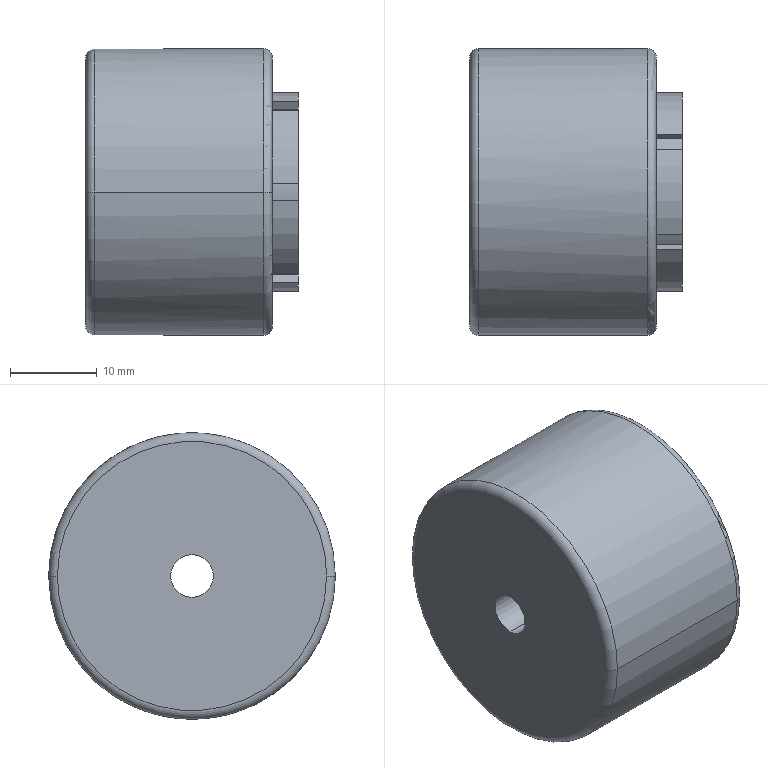Part | STEP file | ZUANZIWAITAO_4_1_2_1_1 | 1 solid | 38 faces | box 24.5 x 33 x 33 mm | volume 18261 mm3 | cylinder 18 | plane 16 | torus 4 | commonest cylinder face diameters 21 x6 23 x6 4.9 x2 17 x2 33 x2
STEP:
#1=CARTESIAN_POINT('',(0.,0.,0.));
#2=DIRECTION('',(0.,0.,1.));
#3=DIRECTION('',(1.,0.,0.));
#4=AXIS2_PLACEMENT_3D('',#1,#2,#3);
#5=CARTESIAN_POINT('',(0.,15.5,0.1054));
#6=VERTEX_POINT('',#5);
#7=CARTESIAN_POINT('',(0.,15.5,0.));
#8=VERTEX_POINT('',#7);
#9=CARTESIAN_POINT('',(0.,0.,0.));
#10=DIRECTION('',(-1.,0.,0.));
#11=DIRECTION('',(0.,1.,0.006802));
#12=AXIS2_PLACEMENT_3D('',#9,#10,#11);
#13=CIRCLE('',#12,15.5);
#14=EDGE_CURVE('',#6,#8,#13,.T.);
#15=ORIENTED_EDGE('',*,*,#14,.F.);
#16=CARTESIAN_POINT('',(0.,-15.5,0.));
#17=VERTEX_POINT('',#16);
#18=CARTESIAN_POINT('',(0.,0.,0.));
#19=DIRECTION('',(1.,0.,0.));
#20=DIRECTION('',(0.,1.,0.006802));
#21=AXIS2_PLACEMENT_3D('',#18,#19,#20);
#22=CIRCLE('',#21,15.5);
#23=EDGE_CURVE('',#6,#17,#22,.T.);
#24=ORIENTED_EDGE('',*,*,#23,.T.);
#25=CARTESIAN_POINT('',(0.,-15.5,-0.1054));
#26=VERTEX_POINT('',#25);
#27=CARTESIAN_POINT('',(0.,0.,0.));
#28=DIRECTION('',(-1.,0.,0.));
#29=DIRECTION('',(0.,-1.,-0.006802));
#30=AXIS2_PLACEMENT_3D('',#27,#28,#29);
#31=CIRCLE('',#30,15.5);
#32=EDGE_CURVE('',#26,#17,#31,.T.);
#33=ORIENTED_EDGE('',*,*,#32,.F.);
#34=CARTESIAN_POINT('',(0.,0.,0.));
#35=DIRECTION('',(1.,0.,0.));
#36=DIRECTION('',(0.,-1.,-0.006802));
#37=AXIS2_PLACEMENT_3D('',#34,#35,#36);
#38=CIRCLE('',#37,15.5);
#39=EDGE_CURVE('',#26,#8,#38,.T.);
#40=ORIENTED_EDGE('',*,*,#39,.T.);
#41=EDGE_LOOP('',(#15,#24,#33,#40));
#42=FACE_OUTER_BOUND('',#41,.F.);
#43=CARTESIAN_POINT('',(0.,0.,2.45));
#44=VERTEX_POINT('',#43);
#45=CARTESIAN_POINT('',(0.,0.,-2.45));
#46=VERTEX_POINT('',#45);
#47=CARTESIAN_POINT('',(0.,0.,0.));
#48=DIRECTION('',(-1.,0.,0.));
#49=DIRECTION('',(0.,0.,1.));
#50=AXIS2_PLACEMENT_3D('',#47,#48,#49);
#51=CIRCLE('',#50,2.45);
#52=EDGE_CURVE('',#44,#46,#51,.T.);
#53=ORIENTED_EDGE('',*,*,#52,.T.);
#54=CARTESIAN_POINT('',(0.,0.,0.));
#55=DIRECTION('',(-1.,0.,0.));
#56=DIRECTION('',(0.,0.,-1.));
#57=AXIS2_PLACEMENT_3D('',#54,#55,#56);
#58=CIRCLE('',#57,2.45);
#59=EDGE_CURVE('',#46,#44,#58,.T.);
#60=ORIENTED_EDGE('',*,*,#59,.T.);
#61=EDGE_LOOP('',(#53,#60));
#62=FACE_BOUND('',#61,.F.);
#63=CARTESIAN_POINT('',(0.,0.,0.));
#64=DIRECTION('',(1.,0.,0.));
#65=DIRECTION('',(0.,-1.,0.));
#66=AXIS2_PLACEMENT_3D('',#63,#64,#65);
#67=PLANE('',#66);
#68=ADVANCED_FACE('',(#42,#62),#67,.F.);
#69=ORIENTED_EDGE('',*,*,#23,.F.);
#70=ORIENTED_EDGE('',*,*,#14,.T.);
#71=CARTESIAN_POINT('',(1.,16.5,0.));
#72=VERTEX_POINT('',#71);
#73=CARTESIAN_POINT('',(1.,15.5,0.));
#74=DIRECTION('',(0.,0.,-1.));
#75=DIRECTION('',(-1.,0.,0.));
#76=AXIS2_PLACEMENT_3D('',#73,#74,#75);
#77=CIRCLE('',#76,1.);
#78=EDGE_CURVE('',#8,#72,#77,.T.);
#79=ORIENTED_EDGE('',*,*,#78,.T.);
#80=CARTESIAN_POINT('',(1.,16.5,0.1122));
#81=VERTEX_POINT('',#80);
#82=CARTESIAN_POINT('',(1.,0.,0.));
#83=DIRECTION('',(1.,0.,0.));
#84=DIRECTION('',(0.,1.,0.));
#85=AXIS2_PLACEMENT_3D('',#82,#83,#84);
#86=CIRCLE('',#85,16.5);
#87=EDGE_CURVE('',#72,#81,#86,.T.);
#88=ORIENTED_EDGE('',*,*,#87,.T.);
#89=CARTESIAN_POINT('',(1.,-16.5,0.));
#90=VERTEX_POINT('',#89);
#91=CARTESIAN_POINT('',(1.,0.,0.));
#92=DIRECTION('',(1.,0.,0.));
#93=DIRECTION('',(0.,1.,0.006802));
#94=AXIS2_PLACEMENT_3D('',#91,#92,#93);
#95=CIRCLE('',#94,16.5);
#96=EDGE_CURVE('',#81,#90,#95,.T.);
#97=ORIENTED_EDGE('',*,*,#96,.T.);
#98=CARTESIAN_POINT('',(1.,-15.5,0.));
#99=DIRECTION('',(0.,0.,1.));
#100=DIRECTION('',(-1.,0.,0.));
#101=AXIS2_PLACEMENT_3D('',#98,#99,#100);
#102=CIRCLE('',#101,1.);
#103=EDGE_CURVE('',#17,#90,#102,.T.);
#104=ORIENTED_EDGE('',*,*,#103,.F.);
#105=EDGE_LOOP('',(#69,#70,#79,#88,#97,#104));
#106=FACE_OUTER_BOUND('',#105,.F.);
#107=CARTESIAN_POINT('',(1.,0.,0.));
#108=DIRECTION('',(1.,0.,0.));
#109=DIRECTION('',(0.,-1.,-0.006802));
#110=AXIS2_PLACEMENT_3D('',#107,#108,#109);
#111=TOROIDAL_SURFACE('',#110,15.5,1.);
#112=ADVANCED_FACE('',(#106),#111,.T.);
#113=ORIENTED_EDGE('',*,*,#39,.F.);
#114=ORIENTED_EDGE('',*,*,#32,.T.);
#115=ORIENTED_EDGE('',*,*,#103,.T.);
#116=CARTESIAN_POINT('',(1.,-16.5,-0.1122));
#117=VERTEX_POINT('',#116);
#118=CARTESIAN_POINT('',(1.,0.,0.));
#119=DIRECTION('',(1.,0.,0.));
#120=DIRECTION('',(0.,-1.,0.));
#121=AXIS2_PLACEMENT_3D('',#118,#119,#120);
#122=CIRCLE('',#121,16.5);
#123=EDGE_CURVE('',#90,#117,#122,.T.);
#124=ORIENTED_EDGE('',*,*,#123,.T.);
#125=CARTESIAN_POINT('',(1.,0.,0.));
#126=DIRECTION('',(1.,0.,0.));
#127=DIRECTION('',(0.,-1.,-0.006802));
#128=AXIS2_PLACEMENT_3D('',#125,#126,#127);
#129=CIRCLE('',#128,16.5);
#130=EDGE_CURVE('',#117,#72,#129,.T.);
#131=ORIENTED_EDGE('',*,*,#130,.T.);
#132=ORIENTED_EDGE('',*,*,#78,.F.);
#133=EDGE_LOOP('',(#113,#114,#115,#124,#131,#132));
#134=FACE_OUTER_BOUND('',#133,.F.);
#135=CARTESIAN_POINT('',(1.,0.,0.));
#136=DIRECTION('',(1.,0.,0.));
#137=DIRECTION('',(0.,1.,0.006802));
#138=AXIS2_PLACEMENT_3D('',#135,#136,#137);
#139=TOROIDAL_SURFACE('',#138,15.5,1.);
#140=ADVANCED_FACE('',(#134),#139,.T.);
#141=CARTESIAN_POINT('',(20.5,16.5,-0.07901));
#142=VERTEX_POINT('',#141);
#143=CARTESIAN_POINT('',(20.5,-16.5,0.));
#144=VERTEX_POINT('',#143);
#145=CARTESIAN_POINT('',(20.5,0.,0.));
#146=DIRECTION('',(-1.,0.,0.));
#147=DIRECTION('',(0.,1.,-0.004788));
#148=AXIS2_PLACEMENT_3D('',#145,#146,#147);
#149=CIRCLE('',#148,16.5);
#150=EDGE_CURVE('',#142,#144,#149,.T.);
#151=ORIENTED_EDGE('',*,*,#150,.F.);
#152=CARTESIAN_POINT('',(20.5,16.5,0.));
#153=VERTEX_POINT('',#152);
#154=CARTESIAN_POINT('',(20.5,0.,0.));
#155=DIRECTION('',(-1.,0.,0.));
#156=DIRECTION('',(0.,1.,0.));
#157=AXIS2_PLACEMENT_3D('',#154,#155,#156);
#158=CIRCLE('',#157,16.5);
#159=EDGE_CURVE('',#153,#142,#158,.T.);
#160=ORIENTED_EDGE('',*,*,#159,.F.);
#161=CARTESIAN_POINT('',(1.,16.5,0.));
#162=DIRECTION('',(1.,0.,0.));
#163=VECTOR('',#162,19.5);
#164=LINE('',#161,#163);
#165=EDGE_CURVE('',#72,#153,#164,.T.);
#166=ORIENTED_EDGE('',*,*,#165,.F.);
#167=ORIENTED_EDGE('',*,*,#130,.F.);
#168=ORIENTED_EDGE('',*,*,#123,.F.);
#169=CARTESIAN_POINT('',(1.,-16.5,0.));
#170=DIRECTION('',(1.,0.,0.));
#171=VECTOR('',#170,19.5);
#172=LINE('',#169,#171);
#173=EDGE_CURVE('',#90,#144,#172,.T.);
#174=ORIENTED_EDGE('',*,*,#173,.T.);
#175=EDGE_LOOP('',(#151,#160,#166,#167,#168,#174));
#176=FACE_OUTER_BOUND('',#175,.F.);
#177=CARTESIAN_POINT('',(0.,0.,0.));
#178=DIRECTION('',(1.,0.,0.));
#179=DIRECTION('',(0.,-1.,0.));
#180=AXIS2_PLACEMENT_3D('',#177,#178,#179);
#181=CYLINDRICAL_SURFACE('',#180,16.5);
#182=ADVANCED_FACE('',(#176),#181,.T.);
#183=CARTESIAN_POINT('',(21.5,15.5,-0.07422));
#184=VERTEX_POINT('',#183);
#185=CARTESIAN_POINT('',(21.5,-15.5,0.));
#186=VERTEX_POINT('',#185);
#187=CARTESIAN_POINT('',(21.5,0.,0.));
#188=DIRECTION('',(-1.,0.,0.));
#189=DIRECTION('',(0.,1.,-0.004788));
#190=AXIS2_PLACEMENT_3D('',#187,#188,#189);
#191=CIRCLE('',#190,15.5);
#192=EDGE_CURVE('',#184,#186,#191,.T.);
#193=ORIENTED_EDGE('',*,*,#192,.F.);
#194=CARTESIAN_POINT('',(21.5,15.5,0.));
#195=VERTEX_POINT('',#194);
#196=CARTESIAN_POINT('',(21.5,0.,0.));
#197=DIRECTION('',(1.,0.,0.));
#198=DIRECTION('',(0.,1.,-0.004788));
#199=AXIS2_PLACEMENT_3D('',#196,#197,#198);
#200=CIRCLE('',#199,15.5);
#201=EDGE_CURVE('',#184,#195,#200,.T.);
#202=ORIENTED_EDGE('',*,*,#201,.T.);
#203=CARTESIAN_POINT('',(20.5,15.5,0.));
#204=DIRECTION('',(0.,0.,1.));
#205=DIRECTION('',(1.,0.,0.));
#206=AXIS2_PLACEMENT_3D('',#203,#204,#205);
#207=CIRCLE('',#206,1.);
#208=EDGE_CURVE('',#195,#153,#207,.T.);
#209=ORIENTED_EDGE('',*,*,#208,.T.);
#210=ORIENTED_EDGE('',*,*,#159,.T.);
#211=ORIENTED_EDGE('',*,*,#150,.T.);
#212=CARTESIAN_POINT('',(20.5,-15.5,0.));
#213=DIRECTION('',(0.,0.,-1.));
#214=DIRECTION('',(1.,0.,0.));
#215=AXIS2_PLACEMENT_3D('',#212,#213,#214);
#216=CIRCLE('',#215,1.);
#217=EDGE_CURVE('',#186,#144,#216,.T.);
#218=ORIENTED_EDGE('',*,*,#217,.F.);
#219=EDGE_LOOP('',(#193,#202,#209,#210,#211,#218));
#220=FACE_OUTER_BOUND('',#219,.F.);
#221=CARTESIAN_POINT('',(20.5,0.,0.));
#222=DIRECTION('',(1.,0.,0.));
#223=DIRECTION('',(0.,-1.,0.004788));
#224=AXIS2_PLACEMENT_3D('',#221,#222,#223);
#225=TOROIDAL_SURFACE('',#224,15.5,1.);
#226=ADVANCED_FACE('',(#220),#225,.T.);
#227=CARTESIAN_POINT('',(21.5,-15.5,0.07422));
#228=VERTEX_POINT('',#227);
#229=CARTESIAN_POINT('',(21.5,0.,0.));
#230=DIRECTION('',(1.,0.,0.));
#231=DIRECTION('',(0.,-1.,0.004788));
#232=AXIS2_PLACEMENT_3D('',#229,#230,#231);
#233=CIRCLE('',#232,15.5);
#234=EDGE_CURVE('',#228,#186,#233,.T.);
#235=ORIENTED_EDGE('',*,*,#234,.F.);
#236=CARTESIAN_POINT('',(21.5,0.,0.));
#237=DIRECTION('',(-1.,0.,0.));
#238=DIRECTION('',(0.,-1.,0.004788));
#239=AXIS2_PLACEMENT_3D('',#236,#237,#238);
#240=CIRCLE('',#239,15.5);
#241=EDGE_CURVE('',#228,#195,#240,.T.);
#242=ORIENTED_EDGE('',*,*,#241,.T.);
#243=ORIENTED_EDGE('',*,*,#201,.F.);
#244=ORIENTED_EDGE('',*,*,#192,.T.);
#245=EDGE_LOOP('',(#235,#242,#243,#244));
#246=FACE_OUTER_BOUND('',#245,.F.);
#247=CARTESIAN_POINT('',(21.5,-6.594,9.422));
#248=VERTEX_POINT('',#247);
#249=CARTESIAN_POINT('',(21.5,-11.456,1.));
#250=VERTEX_POINT('',#249);
#251=CARTESIAN_POINT('',(21.5,0.,0.));
#252=DIRECTION('',(1.,0.,0.));
#253=DIRECTION('',(0.,-0.5734,0.8193));
#254=AXIS2_PLACEMENT_3D('',#251,#252,#253);
#255=CIRCLE('',#254,11.5);
#256=EDGE_CURVE('',#248,#250,#255,.T.);
#257=ORIENTED_EDGE('',*,*,#256,.T.);
#258=CARTESIAN_POINT('',(21.5,-10.452,1.));
#259=VERTEX_POINT('',#258);
#260=CARTESIAN_POINT('',(21.5,-10.452,1.));
#261=DIRECTION('',(0.,-1.,0.));
#262=VECTOR('',#261,1.004);
#263=LINE('',#260,#262);
#264=EDGE_CURVE('',#259,#250,#263,.T.);
#265=ORIENTED_EDGE('',*,*,#264,.F.);
#266=CARTESIAN_POINT('',(21.5,-10.452,-1.));
#267=VERTEX_POINT('',#266);
#268=CARTESIAN_POINT('',(21.5,0.,0.));
#269=DIRECTION('',(1.,0.,0.));
#270=DIRECTION('',(0.,-0.9955,0.09524));
#271=AXIS2_PLACEMENT_3D('',#268,#269,#270);
#272=CIRCLE('',#271,10.5);
#273=EDGE_CURVE('',#259,#267,#272,.T.);
#274=ORIENTED_EDGE('',*,*,#273,.T.);
#275=CARTESIAN_POINT('',(21.5,-11.456,-1.));
#276=VERTEX_POINT('',#275);
#277=CARTESIAN_POINT('',(21.5,-11.456,-1.));
#278=DIRECTION('',(0.,1.,0.));
#279=VECTOR('',#278,1.004);
#280=LINE('',#277,#279);
#281=EDGE_CURVE('',#276,#267,#280,.T.);
#282=ORIENTED_EDGE('',*,*,#281,.F.);
#283=CARTESIAN_POINT('',(21.5,-6.594,-9.422));
#284=VERTEX_POINT('',#283);
#285=CARTESIAN_POINT('',(21.5,0.,0.));
#286=DIRECTION('',(1.,0.,0.));
#287=DIRECTION('',(0.,-0.9962,-0.08696));
#288=AXIS2_PLACEMENT_3D('',#285,#286,#287);
#289=CIRCLE('',#288,11.5);
#290=EDGE_CURVE('',#276,#284,#289,.T.);
#291=ORIENTED_EDGE('',*,*,#290,.T.);
#292=CARTESIAN_POINT('',(21.5,-6.092,-8.552));
#293=VERTEX_POINT('',#292);
#294=CARTESIAN_POINT('',(21.5,-6.594,-9.422));
#295=DIRECTION('',(0.,0.5,0.866));
#296=VECTOR('',#295,1.004);
#297=LINE('',#294,#296);
#298=EDGE_CURVE('',#284,#293,#297,.T.);
#299=ORIENTED_EDGE('',*,*,#298,.T.);
#300=CARTESIAN_POINT('',(21.5,-4.36,-9.552));
#301=VERTEX_POINT('',#300);
#302=CARTESIAN_POINT('',(21.5,0.,0.));
#303=DIRECTION('',(1.,0.,0.));
#304=DIRECTION('',(0.,-0.5802,-0.8145));
#305=AXIS2_PLACEMENT_3D('',#302,#303,#304);
#306=CIRCLE('',#305,10.5);
#307=EDGE_CURVE('',#293,#301,#306,.T.);
#308=ORIENTED_EDGE('',*,*,#307,.T.);
#309=CARTESIAN_POINT('',(21.5,-4.862,-10.422));
#310=VERTEX_POINT('',#309);
#311=CARTESIAN_POINT('',(21.5,-4.36,-9.552));
#312=DIRECTION('',(0.,-0.5,-0.866));
#313=VECTOR('',#312,1.004);
#314=LINE('',#311,#313);
#315=EDGE_CURVE('',#301,#310,#314,.T.);
#316=ORIENTED_EDGE('',*,*,#315,.T.);
#317=CARTESIAN_POINT('',(21.5,4.862,-10.422));
#318=VERTEX_POINT('',#317);
#319=CARTESIAN_POINT('',(21.5,0.,0.));
#320=DIRECTION('',(1.,0.,0.));
#321=DIRECTION('',(0.,-0.4228,-0.9062));
#322=AXIS2_PLACEMENT_3D('',#319,#320,#321);
#323=CIRCLE('',#322,11.5);
#324=EDGE_CURVE('',#310,#318,#323,.T.);
#325=ORIENTED_EDGE('',*,*,#324,.T.);
#326=CARTESIAN_POINT('',(21.5,4.36,-9.552));
#327=VERTEX_POINT('',#326);
#328=CARTESIAN_POINT('',(21.5,4.862,-10.422));
#329=DIRECTION('',(0.,-0.5,0.866));
#330=VECTOR('',#329,1.004);
#331=LINE('',#328,#330);
#332=EDGE_CURVE('',#318,#327,#331,.T.);
#333=ORIENTED_EDGE('',*,*,#332,.T.);
#334=CARTESIAN_POINT('',(21.5,6.092,-8.552));
#335=VERTEX_POINT('',#334);
#336=CARTESIAN_POINT('',(21.5,0.,0.));
#337=DIRECTION('',(1.,0.,0.));
#338=DIRECTION('',(0.,0.4152,-0.9097));
#339=AXIS2_PLACEMENT_3D('',#336,#337,#338);
#340=CIRCLE('',#339,10.5);
#341=EDGE_CURVE('',#327,#335,#340,.T.);
#342=ORIENTED_EDGE('',*,*,#341,.T.);
#343=CARTESIAN_POINT('',(21.5,6.594,-9.422));
#344=VERTEX_POINT('',#343);
#345=CARTESIAN_POINT('',(21.5,6.092,-8.552));
#346=DIRECTION('',(0.,0.5,-0.866));
#347=VECTOR('',#346,1.004);
#348=LINE('',#345,#347);
#349=EDGE_CURVE('',#335,#344,#348,.T.);
#350=ORIENTED_EDGE('',*,*,#349,.T.);
#351=CARTESIAN_POINT('',(21.5,11.456,-1.));
#352=VERTEX_POINT('',#351);
#353=CARTESIAN_POINT('',(21.5,0.,0.));
#354=DIRECTION('',(1.,0.,0.));
#355=DIRECTION('',(0.,0.5734,-0.8193));
#356=AXIS2_PLACEMENT_3D('',#353,#354,#355);
#357=CIRCLE('',#356,11.5);
#358=EDGE_CURVE('',#344,#352,#357,.T.);
#359=ORIENTED_EDGE('',*,*,#358,.T.);
#360=CARTESIAN_POINT('',(21.5,10.452,-1.));
#361=VERTEX_POINT('',#360);
#362=CARTESIAN_POINT('',(21.5,10.452,-1.));
#363=DIRECTION('',(0.,1.,0.));
#364=VECTOR('',#363,1.004);
#365=LINE('',#362,#364);
#366=EDGE_CURVE('',#361,#352,#365,.T.);
#367=ORIENTED_EDGE('',*,*,#366,.F.);
#368=CARTESIAN_POINT('',(21.5,10.452,1.));
#369=VERTEX_POINT('',#368);
#370=CARTESIAN_POINT('',(21.5,0.,0.));
#371=DIRECTION('',(1.,0.,0.));
#372=DIRECTION('',(0.,0.9955,-0.09524));
#373=AXIS2_PLACEMENT_3D('',#370,#371,#372);
#374=CIRCLE('',#373,10.5);
#375=EDGE_CURVE('',#361,#369,#374,.T.);
#376=ORIENTED_EDGE('',*,*,#375,.T.);
#377=CARTESIAN_POINT('',(21.5,11.456,1.));
#378=VERTEX_POINT('',#377);
#379=CARTESIAN_POINT('',(21.5,11.456,1.));
#380=DIRECTION('',(0.,-1.,0.));
#381=VECTOR('',#380,1.004);
#382=LINE('',#379,#381);
#383=EDGE_CURVE('',#378,#369,#382,.T.);
#384=ORIENTED_EDGE('',*,*,#383,.F.);
#385=CARTESIAN_POINT('',(21.5,6.594,9.422));
#386=VERTEX_POINT('',#385);
#387=CARTESIAN_POINT('',(21.5,0.,0.));
#388=DIRECTION('',(1.,0.,0.));
#389=DIRECTION('',(0.,0.9962,0.08696));
#390=AXIS2_PLACEMENT_3D('',#387,#388,#389);
#391=CIRCLE('',#390,11.5);
#392=EDGE_CURVE('',#378,#386,#391,.T.);
#393=ORIENTED_EDGE('',*,*,#392,.T.);
#394=CARTESIAN_POINT('',(21.5,6.092,8.552));
#395=VERTEX_POINT('',#394);
#396=CARTESIAN_POINT('',(21.5,6.594,9.422));
#397=DIRECTION('',(0.,-0.5,-0.866));
#398=VECTOR('',#397,1.004);
#399=LINE('',#396,#398);
#400=EDGE_CURVE('',#386,#395,#399,.T.);
#401=ORIENTED_EDGE('',*,*,#400,.T.);
#402=CARTESIAN_POINT('',(21.5,4.36,9.552));
#403=VERTEX_POINT('',#402);
#404=CARTESIAN_POINT('',(21.5,0.,0.));
#405=DIRECTION('',(1.,0.,0.));
#406=DIRECTION('',(0.,0.5802,0.8145));
#407=AXIS2_PLACEMENT_3D('',#404,#405,#406);
#408=CIRCLE('',#407,10.5);
#409=EDGE_CURVE('',#395,#403,#408,.T.);
#410=ORIENTED_EDGE('',*,*,#409,.T.);
#411=CARTESIAN_POINT('',(21.5,4.862,10.422));
#412=VERTEX_POINT('',#411);
#413=CARTESIAN_POINT('',(21.5,4.36,9.552));
#414=DIRECTION('',(0.,0.5,0.866));
#415=VECTOR('',#414,1.004);
#416=LINE('',#413,#415);
#417=EDGE_CURVE('',#403,#412,#416,.T.);
#418=ORIENTED_EDGE('',*,*,#417,.T.);
#419=CARTESIAN_POINT('',(21.5,-4.862,10.422));
#420=VERTEX_POINT('',#419);
#421=CARTESIAN_POINT('',(21.5,0.,0.));
#422=DIRECTION('',(1.,0.,0.));
#423=DIRECTION('',(0.,0.4228,0.9062));
#424=AXIS2_PLACEMENT_3D('',#421,#422,#423);
#425=CIRCLE('',#424,11.5);
#426=EDGE_CURVE('',#412,#420,#425,.T.);
#427=ORIENTED_EDGE('',*,*,#426,.T.);
#428=CARTESIAN_POINT('',(21.5,-4.36,9.552));
#429=VERTEX_POINT('',#428);
#430=CARTESIAN_POINT('',(21.5,-4.862,10.422));
#431=DIRECTION('',(0.,0.5,-0.866));
#432=VECTOR('',#431,1.004);
#433=LINE('',#430,#432);
#434=EDGE_CURVE('',#420,#429,#433,.T.);
#435=ORIENTED_EDGE('',*,*,#434,.T.);
#436=CARTESIAN_POINT('',(21.5,-6.092,8.552));
#437=VERTEX_POINT('',#436);
#438=CARTESIAN_POINT('',(21.5,0.,0.));
#439=DIRECTION('',(1.,0.,0.));
#440=DIRECTION('',(0.,-0.4152,0.9097));
#441=AXIS2_PLACEMENT_3D('',#438,#439,#440);
#442=CIRCLE('',#441,10.5);
#443=EDGE_CURVE('',#429,#437,#442,.T.);
#444=ORIENTED_EDGE('',*,*,#443,.T.);
#445=CARTESIAN_POINT('',(21.5,-6.092,8.552));
#446=DIRECTION('',(0.,-0.5,0.866));
#447=VECTOR('',#446,1.004);
#448=LINE('',#445,#447);
#449=EDGE_CURVE('',#437,#248,#448,.T.);
#450=ORIENTED_EDGE('',*,*,#449,.T.);
#451=EDGE_LOOP('',(#257,#265,#274,#282,#291,#299,#308,#316,#325,#333,#342,#350,#359,#367,#376,#384,#393,#401,#410,#418,#427,#435,#444,#450));
#452=FACE_BOUND('',#451,.F.);
#453=CARTESIAN_POINT('',(21.5,0.,0.));
#454=DIRECTION('',(1.,0.,0.));
#455=DIRECTION('',(0.,-1.,0.));
#456=AXIS2_PLACEMENT_3D('',#453,#454,#455);
#457=PLANE('',#456);
#458=ADVANCED_FACE('',(#246,#452),#457,.T.);
#459=ORIENTED_EDGE('',*,*,#241,.F.);
#460=ORIENTED_EDGE('',*,*,#234,.T.);
#461=ORIENTED_EDGE('',*,*,#217,.T.);
#462=CARTESIAN_POINT('',(20.5,-16.5,0.07901));
#463=VERTEX_POINT('',#462);
#464=CARTESIAN_POINT('',(20.5,0.,0.));
#465=DIRECTION('',(-1.,0.,0.));
#466=DIRECTION('',(0.,-1.,0.));
#467=AXIS2_PLACEMENT_3D('',#464,#465,#466);
#468=CIRCLE('',#467,16.5);
#469=EDGE_CURVE('',#144,#463,#468,.T.);
#470=ORIENTED_EDGE('',*,*,#469,.T.);
#471=CARTESIAN_POINT('',(20.5,0.,0.));
#472=DIRECTION('',(-1.,0.,0.));
#473=DIRECTION('',(0.,-1.,0.004788));
#474=AXIS2_PLACEMENT_3D('',#471,#472,#473);
#475=CIRCLE('',#474,16.5);
#476=EDGE_CURVE('',#463,#153,#475,.T.);
#477=ORIENTED_EDGE('',*,*,#476,.T.);
#478=ORIENTED_EDGE('',*,*,#208,.F.);
#479=EDGE_LOOP('',(#459,#460,#461,#470,#477,#478));
#480=FACE_OUTER_BOUND('',#479,.F.);
#481=CARTESIAN_POINT('',(20.5,0.,0.));
#482=DIRECTION('',(1.,0.,0.));
#483=DIRECTION('',(0.,1.,-0.004788));
#484=AXIS2_PLACEMENT_3D('',#481,#482,#483);
#485=TOROIDAL_SURFACE('',#484,15.5,1.);
#486=ADVANCED_FACE('',(#480),#485,.T.);
#487=ORIENTED_EDGE('',*,*,#476,.F.);
#488=ORIENTED_EDGE('',*,*,#469,.F.);
#489=ORIENTED_EDGE('',*,*,#173,.F.);
#490=ORIENTED_EDGE('',*,*,#96,.F.);
#491=ORIENTED_EDGE('',*,*,#87,.F.);
#492=ORIENTED_EDGE('',*,*,#165,.T.);
#493=EDGE_LOOP('',(#487,#488,#489,#490,#491,#492));
#494=FACE_OUTER_BOUND('',#493,.F.);
#495=CARTESIAN_POINT('',(0.,0.,0.));
#496=DIRECTION('',(1.,0.,0.));
#497=DIRECTION('',(0.,-1.,0.));
#498=AXIS2_PLACEMENT_3D('',#495,#496,#497);
#499=CYLINDRICAL_SURFACE('',#498,16.5);
#500=ADVANCED_FACE('',(#494),#499,.T.);
#501=CARTESIAN_POINT('',(24.5,-11.456,1.));
#502=VERTEX_POINT('',#501);
#503=CARTESIAN_POINT('',(24.5,-11.456,1.));
#504=DIRECTION('',(-1.,0.,0.));
#505=VECTOR('',#504,3.);
#506=LINE('',#503,#505);
#507=EDGE_CURVE('',#502,#250,#506,.T.);
#508=ORIENTED_EDGE('',*,*,#507,.T.);
#509=ORIENTED_EDGE('',*,*,#256,.F.);
#510=CARTESIAN_POINT('',(24.5,-6.594,9.422));
#511=VERTEX_POINT('',#510);
#512=CARTESIAN_POINT('',(21.5,-6.594,9.422));
#513=DIRECTION('',(1.,0.,0.));
#514=VECTOR('',#513,3.);
#515=LINE('',#512,#514);
#516=EDGE_CURVE('',#248,#511,#515,.T.);
#517=ORIENTED_EDGE('',*,*,#516,.T.);
#518=CARTESIAN_POINT('',(24.5,0.,0.));
#519=DIRECTION('',(-1.,0.,0.));
#520=DIRECTION('',(0.,-0.9962,0.08696));
#521=AXIS2_PLACEMENT_3D('',#518,#519,#520);
#522=CIRCLE('',#521,11.5);
#523=EDGE_CURVE('',#502,#511,#522,.T.);
#524=ORIENTED_EDGE('',*,*,#523,.F.);
#525=EDGE_LOOP('',(#508,#509,#517,#524));
#526=FACE_OUTER_BOUND('',#525,.F.);
#527=CARTESIAN_POINT('',(21.5,0.,0.));
#528=DIRECTION('',(1.,0.,0.));
#529=DIRECTION('',(0.,-1.,0.));
#530=AXIS2_PLACEMENT_3D('',#527,#528,#529);
#531=CYLINDRICAL_SURFACE('',#530,11.5);
#532=ADVANCED_FACE('',(#526),#531,.T.);
#533=CARTESIAN_POINT('',(24.5,-10.452,1.));
#534=VERTEX_POINT('',#533);
#535=CARTESIAN_POINT('',(24.5,-10.452,1.));
#536=DIRECTION('',(0.,-1.,0.));
#537=VECTOR('',#536,1.004);
#538=LINE('',#535,#537);
#539=EDGE_CURVE('',#534,#502,#538,.T.);
#540=ORIENTED_EDGE('',*,*,#539,.F.);
#541=CARTESIAN_POINT('',(21.5,-10.452,1.));
#542=DIRECTION('',(1.,0.,0.));
#543=VECTOR('',#542,3.);
#544=LINE('',#541,#543);
#545=EDGE_CURVE('',#259,#534,#544,.T.);
#546=ORIENTED_EDGE('',*,*,#545,.F.);
#547=ORIENTED_EDGE('',*,*,#264,.T.);
#548=ORIENTED_EDGE('',*,*,#507,.F.);
#549=EDGE_LOOP('',(#540,#546,#547,#548));
#550=FACE_OUTER_BOUND('',#549,.F.);
#551=CARTESIAN_POINT('',(24.5,-10.452,1.));
#552=DIRECTION('',(0.,0.,1.));
#553=DIRECTION('',(0.,-1.,0.));
#554=AXIS2_PLACEMENT_3D('',#551,#552,#553);
#555=PLANE('',#554);
#556=ADVANCED_FACE('',(#550),#555,.F.);
#557=CARTESIAN_POINT('',(24.5,-11.456,-1.));
#558=VERTEX_POINT('',#557);
#559=CARTESIAN_POINT('',(24.5,-10.452,-1.));
#560=VERTEX_POINT('',#559);
#561=CARTESIAN_POINT('',(24.5,-11.456,-1.));
#562=DIRECTION('',(0.,1.,0.));
#563=VECTOR('',#562,1.004);
#564=LINE('',#561,#563);
#565=EDGE_CURVE('',#558,#560,#564,.T.);
#566=ORIENTED_EDGE('',*,*,#565,.T.);
#567=CARTESIAN_POINT('',(24.5,0.,0.));
#568=DIRECTION('',(-1.,0.,0.));
#569=DIRECTION('',(0.,-0.9955,-0.09524));
#570=AXIS2_PLACEMENT_3D('',#567,#568,#569);
#571=CIRCLE('',#570,10.5);
#572=EDGE_CURVE('',#560,#534,#571,.T.);
#573=ORIENTED_EDGE('',*,*,#572,.T.);
#574=ORIENTED_EDGE('',*,*,#539,.T.);
#575=ORIENTED_EDGE('',*,*,#523,.T.);
#576=CARTESIAN_POINT('',(24.5,-6.092,8.552));
#577=VERTEX_POINT('',#576);
#578=CARTESIAN_POINT('',(24.5,-6.594,9.422));
#579=DIRECTION('',(0.,0.5,-0.866));
#580=VECTOR('',#579,1.004);
#581=LINE('',#578,#580);
#582=EDGE_CURVE('',#511,#577,#581,.T.);
#583=ORIENTED_EDGE('',*,*,#582,.T.);
#584=CARTESIAN_POINT('',(24.5,-4.36,9.552));
#585=VERTEX_POINT('',#584);
#586=CARTESIAN_POINT('',(24.5,0.,0.));
#587=DIRECTION('',(-1.,0.,0.));
#588=DIRECTION('',(0.,-0.5802,0.8145));
#589=AXIS2_PLACEMENT_3D('',#586,#587,#588);
#590=CIRCLE('',#589,10.5);
#591=EDGE_CURVE('',#577,#585,#590,.T.);
#592=ORIENTED_EDGE('',*,*,#591,.T.);
#593=CARTESIAN_POINT('',(24.5,-4.862,10.422));
#594=VERTEX_POINT('',#593);
#595=CARTESIAN_POINT('',(24.5,-4.36,9.552));
#596=DIRECTION('',(0.,-0.5,0.866));
#597=VECTOR('',#596,1.004);
#598=LINE('',#595,#597);
#599=EDGE_CURVE('',#585,#594,#598,.T.);
#600=ORIENTED_EDGE('',*,*,#599,.T.);
#601=CARTESIAN_POINT('',(24.5,4.862,10.422));
#602=VERTEX_POINT('',#601);
#603=CARTESIAN_POINT('',(24.5,0.,0.));
#604=DIRECTION('',(-1.,0.,0.));
#605=DIRECTION('',(0.,-0.4228,0.9062));
#606=AXIS2_PLACEMENT_3D('',#603,#604,#605);
#607=CIRCLE('',#606,11.5);
#608=EDGE_CURVE('',#594,#602,#607,.T.);
#609=ORIENTED_EDGE('',*,*,#608,.T.);
#610=CARTESIAN_POINT('',(24.5,4.36,9.552));
#611=VERTEX_POINT('',#610);
#612=CARTESIAN_POINT('',(24.5,4.862,10.422));
#613=DIRECTION('',(0.,-0.5,-0.866));
#614=VECTOR('',#613,1.004);
#615=LINE('',#612,#614);
#616=EDGE_CURVE('',#602,#611,#615,.T.);
#617=ORIENTED_EDGE('',*,*,#616,.T.);
#618=CARTESIAN_POINT('',(24.5,6.092,8.552));
#619=VERTEX_POINT('',#618);
#620=CARTESIAN_POINT('',(24.5,0.,0.));
#621=DIRECTION('',(-1.,0.,0.));
#622=DIRECTION('',(0.,0.4152,0.9097));
#623=AXIS2_PLACEMENT_3D('',#620,#621,#622);
#624=CIRCLE('',#623,10.5);
#625=EDGE_CURVE('',#611,#619,#624,.T.);
#626=ORIENTED_EDGE('',*,*,#625,.T.);
#627=CARTESIAN_POINT('',(24.5,6.594,9.422));
#628=VERTEX_POINT('',#627);
#629=CARTESIAN_POINT('',(24.5,6.092,8.552));
#630=DIRECTION('',(0.,0.5,0.866));
#631=VECTOR('',#630,1.004);
#632=LINE('',#629,#631);
#633=EDGE_CURVE('',#619,#628,#632,.T.);
#634=ORIENTED_EDGE('',*,*,#633,.T.);
#635=CARTESIAN_POINT('',(24.5,11.456,1.));
#636=VERTEX_POINT('',#635);
#637=CARTESIAN_POINT('',(24.5,0.,0.));
#638=DIRECTION('',(-1.,0.,0.));
#639=DIRECTION('',(0.,0.5734,0.8193));
#640=AXIS2_PLACEMENT_3D('',#637,#638,#639);
#641=CIRCLE('',#640,11.5);
#642=EDGE_CURVE('',#628,#636,#641,.T.);
#643=ORIENTED_EDGE('',*,*,#642,.T.);
#644=CARTESIAN_POINT('',(24.5,10.452,1.));
#645=VERTEX_POINT('',#644);
#646=CARTESIAN_POINT('',(24.5,11.456,1.));
#647=DIRECTION('',(0.,-1.,0.));
#648=VECTOR('',#647,1.004);
#649=LINE('',#646,#648);
#650=EDGE_CURVE('',#636,#645,#649,.T.);
#651=ORIENTED_EDGE('',*,*,#650,.T.);
#652=CARTESIAN_POINT('',(24.5,10.452,-1.));
#653=VERTEX_POINT('',#652);
#654=CARTESIAN_POINT('',(24.5,0.,0.));
#655=DIRECTION('',(-1.,0.,0.));
#656=DIRECTION('',(0.,0.9955,0.09524));
#657=AXIS2_PLACEMENT_3D('',#654,#655,#656);
#658=CIRCLE('',#657,10.5);
#659=EDGE_CURVE('',#645,#653,#658,.T.);
#660=ORIENTED_EDGE('',*,*,#659,.T.);
#661=CARTESIAN_POINT('',(24.5,11.456,-1.));
#662=VERTEX_POINT('',#661);
#663=CARTESIAN_POINT('',(24.5,10.452,-1.));
#664=DIRECTION('',(0.,1.,0.));
#665=VECTOR('',#664,1.004);
#666=LINE('',#663,#665);
#667=EDGE_CURVE('',#653,#662,#666,.T.);
#668=ORIENTED_EDGE('',*,*,#667,.T.);
#669=CARTESIAN_POINT('',(24.5,6.594,-9.422));
#670=VERTEX_POINT('',#669);
#671=CARTESIAN_POINT('',(24.5,0.,0.));
#672=DIRECTION('',(-1.,0.,0.));
#673=DIRECTION('',(0.,0.9962,-0.08696));
#674=AXIS2_PLACEMENT_3D('',#671,#672,#673);
#675=CIRCLE('',#674,11.5);
#676=EDGE_CURVE('',#662,#670,#675,.T.);
#677=ORIENTED_EDGE('',*,*,#676,.T.);
#678=CARTESIAN_POINT('',(24.5,6.092,-8.552));
#679=VERTEX_POINT('',#678);
#680=CARTESIAN_POINT('',(24.5,6.594,-9.422));
#681=DIRECTION('',(0.,-0.5,0.866));
#682=VECTOR('',#681,1.004);
#683=LINE('',#680,#682);
#684=EDGE_CURVE('',#670,#679,#683,.T.);
#685=ORIENTED_EDGE('',*,*,#684,.T.);
#686=CARTESIAN_POINT('',(24.5,4.36,-9.552));
#687=VERTEX_POINT('',#686);
#688=CARTESIAN_POINT('',(24.5,0.,0.));
#689=DIRECTION('',(-1.,0.,0.));
#690=DIRECTION('',(0.,0.5802,-0.8145));
#691=AXIS2_PLACEMENT_3D('',#688,#689,#690);
#692=CIRCLE('',#691,10.5);
#693=EDGE_CURVE('',#679,#687,#692,.T.);
#694=ORIENTED_EDGE('',*,*,#693,.T.);
#695=CARTESIAN_POINT('',(24.5,4.862,-10.422));
#696=VERTEX_POINT('',#695);
#697=CARTESIAN_POINT('',(24.5,4.36,-9.552));
#698=DIRECTION('',(0.,0.5,-0.866));
#699=VECTOR('',#698,1.004);
#700=LINE('',#697,#699);
#701=EDGE_CURVE('',#687,#696,#700,.T.);
#702=ORIENTED_EDGE('',*,*,#701,.T.);
#703=CARTESIAN_POINT('',(24.5,-4.862,-10.422));
#704=VERTEX_POINT('',#703);
#705=CARTESIAN_POINT('',(24.5,0.,0.));
#706=DIRECTION('',(-1.,0.,0.));
#707=DIRECTION('',(0.,0.4228,-0.9062));
#708=AXIS2_PLACEMENT_3D('',#705,#706,#707);
#709=CIRCLE('',#708,11.5);
#710=EDGE_CURVE('',#696,#704,#709,.T.);
#711=ORIENTED_EDGE('',*,*,#710,.T.);
#712=CARTESIAN_POINT('',(24.5,-4.36,-9.552));
#713=VERTEX_POINT('',#712);
#714=CARTESIAN_POINT('',(24.5,-4.862,-10.422));
#715=DIRECTION('',(0.,0.5,0.866));
#716=VECTOR('',#715,1.004);
#717=LINE('',#714,#716);
#718=EDGE_CURVE('',#704,#713,#717,.T.);
#719=ORIENTED_EDGE('',*,*,#718,.T.);
#720=CARTESIAN_POINT('',(24.5,-6.092,-8.552));
#721=VERTEX_POINT('',#720);
#722=CARTESIAN_POINT('',(24.5,0.,0.));
#723=DIRECTION('',(-1.,0.,0.));
#724=DIRECTION('',(0.,-0.4152,-0.9097));
#725=AXIS2_PLACEMENT_3D('',#722,#723,#724);
#726=CIRCLE('',#725,10.5);
#727=EDGE_CURVE('',#713,#721,#726,.T.);
#728=ORIENTED_EDGE('',*,*,#727,.T.);
#729=CARTESIAN_POINT('',(24.5,-6.594,-9.422));
#730=VERTEX_POINT('',#729);
#731=CARTESIAN_POINT('',(24.5,-6.092,-8.552));
#732=DIRECTION('',(0.,-0.5,-0.866));
#733=VECTOR('',#732,1.004);
#734=LINE('',#731,#733);
#735=EDGE_CURVE('',#721,#730,#734,.T.);
#736=ORIENTED_EDGE('',*,*,#735,.T.);
#737=CARTESIAN_POINT('',(24.5,0.,0.));
#738=DIRECTION('',(-1.,0.,0.));
#739=DIRECTION('',(0.,-0.5734,-0.8193));
#740=AXIS2_PLACEMENT_3D('',#737,#738,#739);
#741=CIRCLE('',#740,11.5);
#742=EDGE_CURVE('',#730,#558,#741,.T.);
#743=ORIENTED_EDGE('',*,*,#742,.T.);
#744=EDGE_LOOP('',(#566,#573,#574,#575,#583,#592,#600,#609,#617,#626,#634,#643,#651,#660,#668,#677,#685,#694,#702,#711,#719,#728,#736,#743));
#745=FACE_OUTER_BOUND('',#744,.F.);
#746=CARTESIAN_POINT('',(24.5,8.5,0.));
#747=VERTEX_POINT('',#746);
#748=CARTESIAN_POINT('',(24.5,-8.5,0.));
#749=VERTEX_POINT('',#748);
#750=CARTESIAN_POINT('',(24.5,0.,0.));
#751=DIRECTION('',(1.,0.,0.));
#752=DIRECTION('',(0.,1.,0.));
#753=AXIS2_PLACEMENT_3D('',#750,#751,#752);
#754=CIRCLE('',#753,8.5);
#755=EDGE_CURVE('',#747,#749,#754,.T.);
#756=ORIENTED_EDGE('',*,*,#755,.T.);
#757=CARTESIAN_POINT('',(24.5,0.,0.));
#758=DIRECTION('',(1.,0.,0.));
#759=DIRECTION('',(0.,-1.,0.));
#760=AXIS2_PLACEMENT_3D('',#757,#758,#759);
#761=CIRCLE('',#760,8.5);
#762=EDGE_CURVE('',#749,#747,#761,.T.);
#763=ORIENTED_EDGE('',*,*,#762,.T.);
#764=EDGE_LOOP('',(#756,#763));
#765=FACE_BOUND('',#764,.F.);
#766=CARTESIAN_POINT('',(24.5,0.,0.));
#767=DIRECTION('',(1.,0.,0.));
#768=DIRECTION('',(0.,-1.,0.));
#769=AXIS2_PLACEMENT_3D('',#766,#767,#768);
#770=PLANE('',#769);
#771=ADVANCED_FACE('',(#745,#765),#770,.T.);
#772=ORIENTED_EDGE('',*,*,#565,.F.);
#773=CARTESIAN_POINT('',(21.5,-11.456,-1.));
#774=DIRECTION('',(1.,0.,0.));
#775=VECTOR('',#774,3.);
#776=LINE('',#773,#775);
#777=EDGE_CURVE('',#276,#558,#776,.T.);
#778=ORIENTED_EDGE('',*,*,#777,.F.);
#779=ORIENTED_EDGE('',*,*,#281,.T.);
#780=CARTESIAN_POINT('',(24.5,-10.452,-1.));
#781=DIRECTION('',(-1.,0.,0.));
#782=VECTOR('',#781,3.);
#783=LINE('',#780,#782);
#784=EDGE_CURVE('',#560,#267,#783,.T.);
#785=ORIENTED_EDGE('',*,*,#784,.F.);
#786=EDGE_LOOP('',(#772,#778,#779,#785));
#787=FACE_OUTER_BOUND('',#786,.F.);
#788=CARTESIAN_POINT('',(24.5,-11.456,-1.));
#789=DIRECTION('',(0.,0.,-1.));
#790=DIRECTION('',(0.,1.,0.));
#791=AXIS2_PLACEMENT_3D('',#788,#789,#790);
#792=PLANE('',#791);
#793=ADVANCED_FACE('',(#787),#792,.F.);
#794=ORIENTED_EDGE('',*,*,#777,.T.);
#795=ORIENTED_EDGE('',*,*,#742,.F.);
#796=CARTESIAN_POINT('',(24.5,-6.594,-9.422));
#797=DIRECTION('',(-1.,0.,0.));
#798=VECTOR('',#797,3.);
#799=LINE('',#796,#798);
#800=EDGE_CURVE('',#730,#284,#799,.T.);
#801=ORIENTED_EDGE('',*,*,#800,.T.);
#802=ORIENTED_EDGE('',*,*,#290,.F.);
#803=EDGE_LOOP('',(#794,#795,#801,#802));
#804=FACE_OUTER_BOUND('',#803,.F.);
#805=CARTESIAN_POINT('',(21.5,0.,0.));
#806=DIRECTION('',(1.,0.,0.));
#807=DIRECTION('',(0.,-1.,0.));
#808=AXIS2_PLACEMENT_3D('',#805,#806,#807);
#809=CYLINDRICAL_SURFACE('',#808,11.5);
#810=ADVANCED_FACE('',(#804),#809,.T.);
#811=ORIENTED_EDGE('',*,*,#735,.F.);
#812=CARTESIAN_POINT('',(21.5,-6.092,-8.552));
#813=DIRECTION('',(1.,0.,0.));
#814=VECTOR('',#813,3.);
#815=LINE('',#812,#814);
#816=EDGE_CURVE('',#293,#721,#815,.T.);
#817=ORIENTED_EDGE('',*,*,#816,.F.);
#818=ORIENTED_EDGE('',*,*,#298,.F.);
#819=ORIENTED_EDGE('',*,*,#800,.F.);
#820=EDGE_LOOP('',(#811,#817,#818,#819));
#821=FACE_OUTER_BOUND('',#820,.F.);
#822=CARTESIAN_POINT('',(24.5,-6.092,-8.552));
#823=DIRECTION('',(0.,-0.866,0.5));
#824=DIRECTION('',(0.,-0.5,-0.866));
#825=AXIS2_PLACEMENT_3D('',#822,#823,#824);
#826=PLANE('',#825);
#827=ADVANCED_FACE('',(#821),#826,.F.);
#828=ORIENTED_EDGE('',*,*,#727,.F.);
#829=CARTESIAN_POINT('',(24.5,-4.36,-9.552));
#830=DIRECTION('',(-1.,0.,0.));
#831=VECTOR('',#830,3.);
#832=LINE('',#829,#831);
#833=EDGE_CURVE('',#713,#301,#832,.T.);
#834=ORIENTED_EDGE('',*,*,#833,.T.);
#835=ORIENTED_EDGE('',*,*,#307,.F.);
#836=ORIENTED_EDGE('',*,*,#816,.T.);
#837=EDGE_LOOP('',(#828,#834,#835,#836));
#838=FACE_OUTER_BOUND('',#837,.F.);
#839=CARTESIAN_POINT('',(24.5,0.,0.));
#840=DIRECTION('',(1.,0.,0.));
#841=DIRECTION('',(0.,-1.,0.));
#842=AXIS2_PLACEMENT_3D('',#839,#840,#841);
#843=CYLINDRICAL_SURFACE('',#842,10.5);
#844=ADVANCED_FACE('',(#838),#843,.T.);
#845=ORIENTED_EDGE('',*,*,#718,.F.);
#846=CARTESIAN_POINT('',(21.5,-4.862,-10.422));
#847=DIRECTION('',(1.,0.,0.));
#848=VECTOR('',#847,3.);
#849=LINE('',#846,#848);
#850=EDGE_CURVE('',#310,#704,#849,.T.);
#851=ORIENTED_EDGE('',*,*,#850,.F.);
#852=ORIENTED_EDGE('',*,*,#315,.F.);
#853=ORIENTED_EDGE('',*,*,#833,.F.);
#854=EDGE_LOOP('',(#845,#851,#852,#853));
#855=FACE_OUTER_BOUND('',#854,.F.);
#856=CARTESIAN_POINT('',(24.5,-4.862,-10.422));
#857=DIRECTION('',(0.,0.866,-0.5));
#858=DIRECTION('',(0.,0.5,0.866));
#859=AXIS2_PLACEMENT_3D('',#856,#857,#858);
#860=PLANE('',#859);
#861=ADVANCED_FACE('',(#855),#860,.F.);
#862=CARTESIAN_POINT('',(24.5,4.862,-10.422));
#863=DIRECTION('',(-1.,0.,0.));
#864=VECTOR('',#863,3.);
#865=LINE('',#862,#864);
#866=EDGE_CURVE('',#696,#318,#865,.T.);
#867=ORIENTED_EDGE('',*,*,#866,.T.);
#868=ORIENTED_EDGE('',*,*,#324,.F.);
#869=ORIENTED_EDGE('',*,*,#850,.T.);
#870=ORIENTED_EDGE('',*,*,#710,.F.);
#871=EDGE_LOOP('',(#867,#868,#869,#870));
#872=FACE_OUTER_BOUND('',#871,.F.);
#873=CARTESIAN_POINT('',(21.5,0.,0.));
#874=DIRECTION('',(1.,0.,0.));
#875=DIRECTION('',(0.,-1.,0.));
#876=AXIS2_PLACEMENT_3D('',#873,#874,#875);
#877=CYLINDRICAL_SURFACE('',#876,11.5);
#878=ADVANCED_FACE('',(#872),#877,.T.);
#879=ORIENTED_EDGE('',*,*,#701,.F.);
#880=CARTESIAN_POINT('',(21.5,4.36,-9.552));
#881=DIRECTION('',(1.,0.,0.));
#882=VECTOR('',#881,3.);
#883=LINE('',#880,#882);
#884=EDGE_CURVE('',#327,#687,#883,.T.);
#885=ORIENTED_EDGE('',*,*,#884,.F.);
#886=ORIENTED_EDGE('',*,*,#332,.F.);
#887=ORIENTED_EDGE('',*,*,#866,.F.);
#888=EDGE_LOOP('',(#879,#885,#886,#887));
#889=FACE_OUTER_BOUND('',#888,.F.);
#890=CARTESIAN_POINT('',(24.5,4.36,-9.552));
#891=DIRECTION('',(0.,-0.866,-0.5));
#892=DIRECTION('',(0.,0.5,-0.866));
#893=AXIS2_PLACEMENT_3D('',#890,#891,#892);
#894=PLANE('',#893);
#895=ADVANCED_FACE('',(#889),#894,.F.);
#896=ORIENTED_EDGE('',*,*,#693,.F.);
#897=CARTESIAN_POINT('',(24.5,6.092,-8.552));
#898=DIRECTION('',(-1.,0.,0.));
#899=VECTOR('',#898,3.);
#900=LINE('',#897,#899);
#901=EDGE_CURVE('',#679,#335,#900,.T.);
#902=ORIENTED_EDGE('',*,*,#901,.T.);
#903=ORIENTED_EDGE('',*,*,#341,.F.);
#904=ORIENTED_EDGE('',*,*,#884,.T.);
#905=EDGE_LOOP('',(#896,#902,#903,#904));
#906=FACE_OUTER_BOUND('',#905,.F.);
#907=CARTESIAN_POINT('',(24.5,0.,0.));
#908=DIRECTION('',(1.,0.,0.));
#909=DIRECTION('',(0.,-0.5,-0.866));
#910=AXIS2_PLACEMENT_3D('',#907,#908,#909);
#911=CYLINDRICAL_SURFACE('',#910,10.5);
#912=ADVANCED_FACE('',(#906),#911,.T.);
#913=ORIENTED_EDGE('',*,*,#684,.F.);
#914=CARTESIAN_POINT('',(21.5,6.594,-9.422));
#915=DIRECTION('',(1.,0.,0.));
#916=VECTOR('',#915,3.);
#917=LINE('',#914,#916);
#918=EDGE_CURVE('',#344,#670,#917,.T.);
#919=ORIENTED_EDGE('',*,*,#918,.F.);
#920=ORIENTED_EDGE('',*,*,#349,.F.);
#921=ORIENTED_EDGE('',*,*,#901,.F.);
#922=EDGE_LOOP('',(#913,#919,#920,#921));
#923=FACE_OUTER_BOUND('',#922,.F.);
#924=CARTESIAN_POINT('',(24.5,6.594,-9.422));
#925=DIRECTION('',(0.,0.866,0.5));
#926=DIRECTION('',(0.,-0.5,0.866));
#927=AXIS2_PLACEMENT_3D('',#924,#925,#926);
#928=PLANE('',#927);
#929=ADVANCED_FACE('',(#923),#928,.F.);
#930=CARTESIAN_POINT('',(24.5,11.456,-1.));
#931=DIRECTION('',(-1.,0.,0.));
#932=VECTOR('',#931,3.);
#933=LINE('',#930,#932);
#934=EDGE_CURVE('',#662,#352,#933,.T.);
#935=ORIENTED_EDGE('',*,*,#934,.T.);
#936=ORIENTED_EDGE('',*,*,#358,.F.);
#937=ORIENTED_EDGE('',*,*,#918,.T.);
#938=ORIENTED_EDGE('',*,*,#676,.F.);
#939=EDGE_LOOP('',(#935,#936,#937,#938));
#940=FACE_OUTER_BOUND('',#939,.F.);
#941=CARTESIAN_POINT('',(21.5,0.,0.));
#942=DIRECTION('',(1.,0.,0.));
#943=DIRECTION('',(0.,-1.,0.));
#944=AXIS2_PLACEMENT_3D('',#941,#942,#943);
#945=CYLINDRICAL_SURFACE('',#944,11.5);
#946=ADVANCED_FACE('',(#940),#945,.T.);
#947=ORIENTED_EDGE('',*,*,#667,.F.);
#948=CARTESIAN_POINT('',(21.5,10.452,-1.));
#949=DIRECTION('',(1.,0.,0.));
#950=VECTOR('',#949,3.);
#951=LINE('',#948,#950);
#952=EDGE_CURVE('',#361,#653,#951,.T.);
#953=ORIENTED_EDGE('',*,*,#952,.F.);
#954=ORIENTED_EDGE('',*,*,#366,.T.);
#955=ORIENTED_EDGE('',*,*,#934,.F.);
#956=EDGE_LOOP('',(#947,#953,#954,#955));
#957=FACE_OUTER_BOUND('',#956,.F.);
#958=CARTESIAN_POINT('',(24.5,10.452,-1.));
#959=DIRECTION('',(0.,0.,-1.));
#960=DIRECTION('',(0.,1.,0.));
#961=AXIS2_PLACEMENT_3D('',#958,#959,#960);
#962=PLANE('',#961);
#963=ADVANCED_FACE('',(#957),#962,.F.);
#964=ORIENTED_EDGE('',*,*,#659,.F.);
#965=CARTESIAN_POINT('',(24.5,10.452,1.));
#966=DIRECTION('',(-1.,0.,0.));
#967=VECTOR('',#966,3.);
#968=LINE('',#965,#967);
#969=EDGE_CURVE('',#645,#369,#968,.T.);
#970=ORIENTED_EDGE('',*,*,#969,.T.);
#971=ORIENTED_EDGE('',*,*,#375,.F.);
#972=ORIENTED_EDGE('',*,*,#952,.T.);
#973=EDGE_LOOP('',(#964,#970,#971,#972));
#974=FACE_OUTER_BOUND('',#973,.F.);
#975=CARTESIAN_POINT('',(24.5,0.,0.));
#976=DIRECTION('',(1.,0.,0.));
#977=DIRECTION('',(0.,0.5,-0.866));
#978=AXIS2_PLACEMENT_3D('',#975,#976,#977);
#979=CYLINDRICAL_SURFACE('',#978,10.5);
#980=ADVANCED_FACE('',(#974),#979,.T.);
#981=ORIENTED_EDGE('',*,*,#650,.F.);
#982=CARTESIAN_POINT('',(21.5,11.456,1.));
#983=DIRECTION('',(1.,0.,0.));
#984=VECTOR('',#983,3.);
#985=LINE('',#982,#984);
#986=EDGE_CURVE('',#378,#636,#985,.T.);
#987=ORIENTED_EDGE('',*,*,#986,.F.);
#988=ORIENTED_EDGE('',*,*,#383,.T.);
#989=ORIENTED_EDGE('',*,*,#969,.F.);
#990=EDGE_LOOP('',(#981,#987,#988,#989));
#991=FACE_OUTER_BOUND('',#990,.F.);
#992=CARTESIAN_POINT('',(24.5,11.456,1.));
#993=DIRECTION('',(0.,0.,1.));
#994=DIRECTION('',(0.,-1.,0.));
#995=AXIS2_PLACEMENT_3D('',#992,#993,#994);
#996=PLANE('',#995);
#997=ADVANCED_FACE('',(#991),#996,.F.);
#998=CARTESIAN_POINT('',(24.5,6.594,9.422));
#999=DIRECTION('',(-1.,0.,0.));
#1000=VECTOR('',#999,3.);
#1001=LINE('',#998,#1000);
#1002=EDGE_CURVE('',#628,#386,#1001,.T.);
#1003=ORIENTED_EDGE('',*,*,#1002,.T.);
#1004=ORIENTED_EDGE('',*,*,#392,.F.);
#1005=ORIENTED_EDGE('',*,*,#986,.T.);
#1006=ORIENTED_EDGE('',*,*,#642,.F.);
#1007=EDGE_LOOP('',(#1003,#1004,#1005,#1006));
#1008=FACE_OUTER_BOUND('',#1007,.F.);
#1009=CARTESIAN_POINT('',(21.5,0.,0.));
#1010=DIRECTION('',(1.,0.,0.));
#1011=DIRECTION('',(0.,-1.,0.));
#1012=AXIS2_PLACEMENT_3D('',#1009,#1010,#1011);
#1013=CYLINDRICAL_SURFACE('',#1012,11.5);
#1014=ADVANCED_FACE('',(#1008),#1013,.T.);
#1015=ORIENTED_EDGE('',*,*,#633,.F.);
#1016=CARTESIAN_POINT('',(21.5,6.092,8.552));
#1017=DIRECTION('',(1.,0.,0.));
#1018=VECTOR('',#1017,3.);
#1019=LINE('',#1016,#1018);
#1020=EDGE_CURVE('',#395,#619,#1019,.T.);
#1021=ORIENTED_EDGE('',*,*,#1020,.F.);
#1022=ORIENTED_EDGE('',*,*,#400,.F.);
#1023=ORIENTED_EDGE('',*,*,#1002,.F.);
#1024=EDGE_LOOP('',(#1015,#1021,#1022,#1023));
#1025=FACE_OUTER_BOUND('',#1024,.F.);
#1026=CARTESIAN_POINT('',(24.5,6.092,8.552));
#1027=DIRECTION('',(0.,0.866,-0.5));
#1028=DIRECTION('',(0.,0.5,0.866));
#1029=AXIS2_PLACEMENT_3D('',#1026,#1027,#1028);
#1030=PLANE('',#1029);
#1031=ADVANCED_FACE('',(#1025),#1030,.F.);
#1032=ORIENTED_EDGE('',*,*,#625,.F.);
#1033=CARTESIAN_POINT('',(24.5,4.36,9.552));
#1034=DIRECTION('',(-1.,0.,0.));
#1035=VECTOR('',#1034,3.);
#1036=LINE('',#1033,#1035);
#1037=EDGE_CURVE('',#611,#403,#1036,.T.);
#1038=ORIENTED_EDGE('',*,*,#1037,.T.);
#1039=ORIENTED_EDGE('',*,*,#409,.F.);
#1040=ORIENTED_EDGE('',*,*,#1020,.T.);
#1041=EDGE_LOOP('',(#1032,#1038,#1039,#1040));
#1042=FACE_OUTER_BOUND('',#1041,.F.);
#1043=CARTESIAN_POINT('',(24.5,0.,0.));
#1044=DIRECTION('',(1.,0.,0.));
#1045=DIRECTION('',(0.,1.,0.));
#1046=AXIS2_PLACEMENT_3D('',#1043,#1044,#1045);
#1047=CYLINDRICAL_SURFACE('',#1046,10.5);
#1048=ADVANCED_FACE('',(#1042),#1047,.T.);
#1049=ORIENTED_EDGE('',*,*,#616,.F.);
#1050=CARTESIAN_POINT('',(21.5,4.862,10.422));
#1051=DIRECTION('',(1.,0.,0.));
#1052=VECTOR('',#1051,3.);
#1053=LINE('',#1050,#1052);
#1054=EDGE_CURVE('',#412,#602,#1053,.T.);
#1055=ORIENTED_EDGE('',*,*,#1054,.F.);
#1056=ORIENTED_EDGE('',*,*,#417,.F.);
#1057=ORIENTED_EDGE('',*,*,#1037,.F.);
#1058=EDGE_LOOP('',(#1049,#1055,#1056,#1057));
#1059=FACE_OUTER_BOUND('',#1058,.F.);
#1060=CARTESIAN_POINT('',(24.5,4.862,10.422));
#1061=DIRECTION('',(0.,-0.866,0.5));
#1062=DIRECTION('',(0.,-0.5,-0.866));
#1063=AXIS2_PLACEMENT_3D('',#1060,#1061,#1062);
#1064=PLANE('',#1063);
#1065=ADVANCED_FACE('',(#1059),#1064,.F.);
#1066=CARTESIAN_POINT('',(24.5,-4.862,10.422));
#1067=DIRECTION('',(-1.,0.,0.));
#1068=VECTOR('',#1067,3.);
#1069=LINE('',#1066,#1068);
#1070=EDGE_CURVE('',#594,#420,#1069,.T.);
#1071=ORIENTED_EDGE('',*,*,#1070,.T.);
#1072=ORIENTED_EDGE('',*,*,#426,.F.);
#1073=ORIENTED_EDGE('',*,*,#1054,.T.);
#1074=ORIENTED_EDGE('',*,*,#608,.F.);
#1075=EDGE_LOOP('',(#1071,#1072,#1073,#1074));
#1076=FACE_OUTER_BOUND('',#1075,.F.);
#1077=CARTESIAN_POINT('',(21.5,0.,0.));
#1078=DIRECTION('',(1.,0.,0.));
#1079=DIRECTION('',(0.,-1.,0.));
#1080=AXIS2_PLACEMENT_3D('',#1077,#1078,#1079);
#1081=CYLINDRICAL_SURFACE('',#1080,11.5);
#1082=ADVANCED_FACE('',(#1076),#1081,.T.);
#1083=ORIENTED_EDGE('',*,*,#599,.F.);
#1084=CARTESIAN_POINT('',(21.5,-4.36,9.552));
#1085=DIRECTION('',(1.,0.,0.));
#1086=VECTOR('',#1085,3.);
#1087=LINE('',#1084,#1086);
#1088=EDGE_CURVE('',#429,#585,#1087,.T.);
#1089=ORIENTED_EDGE('',*,*,#1088,.F.);
#1090=ORIENTED_EDGE('',*,*,#434,.F.);
#1091=ORIENTED_EDGE('',*,*,#1070,.F.);
#1092=EDGE_LOOP('',(#1083,#1089,#1090,#1091));
#1093=FACE_OUTER_BOUND('',#1092,.F.);
#1094=CARTESIAN_POINT('',(24.5,-4.36,9.552));
#1095=DIRECTION('',(0.,0.866,0.5));
#1096=DIRECTION('',(0.,-0.5,0.866));
#1097=AXIS2_PLACEMENT_3D('',#1094,#1095,#1096);
#1098=PLANE('',#1097);
#1099=ADVANCED_FACE('',(#1093),#1098,.F.);
#1100=ORIENTED_EDGE('',*,*,#591,.F.);
#1101=CARTESIAN_POINT('',(24.5,-6.092,8.552));
#1102=DIRECTION('',(-1.,0.,0.));
#1103=VECTOR('',#1102,3.);
#1104=LINE('',#1101,#1103);
#1105=EDGE_CURVE('',#577,#437,#1104,.T.);
#1106=ORIENTED_EDGE('',*,*,#1105,.T.);
#1107=ORIENTED_EDGE('',*,*,#443,.F.);
#1108=ORIENTED_EDGE('',*,*,#1088,.T.);
#1109=EDGE_LOOP('',(#1100,#1106,#1107,#1108));
#1110=FACE_OUTER_BOUND('',#1109,.F.);
#1111=CARTESIAN_POINT('',(24.5,0.,0.));
#1112=DIRECTION('',(1.,0.,0.));
#1113=DIRECTION('',(0.,0.5,0.866));
#1114=AXIS2_PLACEMENT_3D('',#1111,#1112,#1113);
#1115=CYLINDRICAL_SURFACE('',#1114,10.5);
#1116=ADVANCED_FACE('',(#1110),#1115,.T.);
#1117=ORIENTED_EDGE('',*,*,#582,.F.);
#1118=ORIENTED_EDGE('',*,*,#516,.F.);
#1119=ORIENTED_EDGE('',*,*,#449,.F.);
#1120=ORIENTED_EDGE('',*,*,#1105,.F.);
#1121=EDGE_LOOP('',(#1117,#1118,#1119,#1120));
#1122=FACE_OUTER_BOUND('',#1121,.F.);
#1123=CARTESIAN_POINT('',(24.5,-6.594,9.422));
#1124=DIRECTION('',(0.,-0.866,-0.5));
#1125=DIRECTION('',(0.,0.5,-0.866));
#1126=AXIS2_PLACEMENT_3D('',#1123,#1124,#1125);
#1127=PLANE('',#1126);
#1128=ADVANCED_FACE('',(#1122),#1127,.F.);
#1129=ORIENTED_EDGE('',*,*,#572,.F.);
#1130=ORIENTED_EDGE('',*,*,#784,.T.);
#1131=ORIENTED_EDGE('',*,*,#273,.F.);
#1132=ORIENTED_EDGE('',*,*,#545,.T.);
#1133=EDGE_LOOP('',(#1129,#1130,#1131,#1132));
#1134=FACE_OUTER_BOUND('',#1133,.F.);
#1135=CARTESIAN_POINT('',(24.5,0.,0.));
#1136=DIRECTION('',(1.,0.,0.));
#1137=DIRECTION('',(0.,-0.5,0.866));
#1138=AXIS2_PLACEMENT_3D('',#1135,#1136,#1137);
#1139=CYLINDRICAL_SURFACE('',#1138,10.5);
#1140=ADVANCED_FACE('',(#1134),#1139,.T.);
#1141=CARTESIAN_POINT('',(20.5,8.5,0.));
#1142=VERTEX_POINT('',#1141);
#1143=CARTESIAN_POINT('',(24.5,8.5,0.));
#1144=DIRECTION('',(-1.,0.,0.));
#1145=VECTOR('',#1144,4.);
#1146=LINE('',#1143,#1145);
#1147=EDGE_CURVE('',#747,#1142,#1146,.T.);
#1148=ORIENTED_EDGE('',*,*,#1147,.T.);
#1149=CARTESIAN_POINT('',(20.5,-8.5,0.));
#1150=VERTEX_POINT('',#1149);
#1151=CARTESIAN_POINT('',(20.5,0.,0.));
#1152=DIRECTION('',(-1.,0.,0.));
#1153=DIRECTION('',(0.,-1.,0.));
#1154=AXIS2_PLACEMENT_3D('',#1151,#1152,#1153);
#1155=CIRCLE('',#1154,8.5);
#1156=EDGE_CURVE('',#1150,#1142,#1155,.T.);
#1157=ORIENTED_EDGE('',*,*,#1156,.F.);
#1158=CARTESIAN_POINT('',(20.5,-8.5,0.));
#1159=DIRECTION('',(1.,0.,0.));
#1160=VECTOR('',#1159,4.);
#1161=LINE('',#1158,#1160);
#1162=EDGE_CURVE('',#1150,#749,#1161,.T.);
#1163=ORIENTED_EDGE('',*,*,#1162,.T.);
#1164=ORIENTED_EDGE('',*,*,#755,.F.);
#1165=EDGE_LOOP('',(#1148,#1157,#1163,#1164));
#1166=FACE_OUTER_BOUND('',#1165,.F.);
#1167=CARTESIAN_POINT('',(21.5,0.,0.));
#1168=DIRECTION('',(1.,0.,0.));
#1169=DIRECTION('',(0.,-1.,0.));
#1170=AXIS2_PLACEMENT_3D('',#1167,#1168,#1169);
#1171=CYLINDRICAL_SURFACE('',#1170,8.5);
#1172=ADVANCED_FACE('',(#1166),#1171,.F.);
#1173=ORIENTED_EDGE('',*,*,#1162,.F.);
#1174=CARTESIAN_POINT('',(20.5,0.,0.));
#1175=DIRECTION('',(-1.,0.,0.));
#1176=DIRECTION('',(0.,1.,0.));
#1177=AXIS2_PLACEMENT_3D('',#1174,#1175,#1176);
#1178=CIRCLE('',#1177,8.5);
#1179=EDGE_CURVE('',#1142,#1150,#1178,.T.);
#1180=ORIENTED_EDGE('',*,*,#1179,.F.);
#1181=ORIENTED_EDGE('',*,*,#1147,.F.);
#1182=ORIENTED_EDGE('',*,*,#762,.F.);
#1183=EDGE_LOOP('',(#1173,#1180,#1181,#1182));
#1184=FACE_OUTER_BOUND('',#1183,.F.);
#1185=CARTESIAN_POINT('',(21.5,0.,0.));
#1186=DIRECTION('',(1.,0.,0.));
#1187=DIRECTION('',(0.,-1.,0.));
#1188=AXIS2_PLACEMENT_3D('',#1185,#1186,#1187);
#1189=CYLINDRICAL_SURFACE('',#1188,8.5);
#1190=ADVANCED_FACE('',(#1184),#1189,.F.);
#1191=ORIENTED_EDGE('',*,*,#1179,.T.);
#1192=ORIENTED_EDGE('',*,*,#1156,.T.);
#1193=EDGE_LOOP('',(#1191,#1192));
#1194=FACE_OUTER_BOUND('',#1193,.F.);
#1195=CARTESIAN_POINT('',(20.5,0.,-2.45));
#1196=VERTEX_POINT('',#1195);
#1197=CARTESIAN_POINT('',(20.5,0.,2.45));
#1198=VERTEX_POINT('',#1197);
#1199=CARTESIAN_POINT('',(20.5,0.,0.));
#1200=DIRECTION('',(1.,0.,0.));
#1201=DIRECTION('',(0.,0.,-1.));
#1202=AXIS2_PLACEMENT_3D('',#1199,#1200,#1201);
#1203=CIRCLE('',#1202,2.45);
#1204=EDGE_CURVE('',#1196,#1198,#1203,.T.);
#1205=ORIENTED_EDGE('',*,*,#1204,.T.);
#1206=CARTESIAN_POINT('',(20.5,0.,0.));
#1207=DIRECTION('',(1.,0.,0.));
#1208=DIRECTION('',(0.,0.,1.));
#1209=AXIS2_PLACEMENT_3D('',#1206,#1207,#1208);
#1210=CIRCLE('',#1209,2.45);
#1211=EDGE_CURVE('',#1198,#1196,#1210,.T.);
#1212=ORIENTED_EDGE('',*,*,#1211,.T.);
#1213=EDGE_LOOP('',(#1205,#1212));
#1214=FACE_BOUND('',#1213,.F.);
#1215=CARTESIAN_POINT('',(20.5,0.,0.));
#1216=DIRECTION('',(1.,0.,0.));
#1217=DIRECTION('',(0.,-1.,0.));
#1218=AXIS2_PLACEMENT_3D('',#1215,#1216,#1217);
#1219=PLANE('',#1218);
#1220=ADVANCED_FACE('',(#1194,#1214),#1219,.T.);
#1221=ORIENTED_EDGE('',*,*,#52,.F.);
#1222=CARTESIAN_POINT('',(0.,0.,2.45));
#1223=DIRECTION('',(1.,0.,0.));
#1224=VECTOR('',#1223,20.5);
#1225=LINE('',#1222,#1224);
#1226=EDGE_CURVE('',#44,#1198,#1225,.T.);
#1227=ORIENTED_EDGE('',*,*,#1226,.T.);
#1228=ORIENTED_EDGE('',*,*,#1204,.F.);
#1229=CARTESIAN_POINT('',(0.,0.,-2.45));
#1230=DIRECTION('',(1.,0.,0.));
#1231=VECTOR('',#1230,20.5);
#1232=LINE('',#1229,#1231);
#1233=EDGE_CURVE('',#46,#1196,#1232,.T.);
#1234=ORIENTED_EDGE('',*,*,#1233,.F.);
#1235=EDGE_LOOP('',(#1221,#1227,#1228,#1234));
#1236=FACE_OUTER_BOUND('',#1235,.F.);
#1237=CARTESIAN_POINT('',(0.,0.,0.));
#1238=DIRECTION('',(-1.,0.,0.));
#1239=DIRECTION('',(0.,0.,1.));
#1240=AXIS2_PLACEMENT_3D('',#1237,#1238,#1239);
#1241=CYLINDRICAL_SURFACE('',#1240,2.45);
#1242=ADVANCED_FACE('',(#1236),#1241,.F.);
#1243=ORIENTED_EDGE('',*,*,#59,.F.);
#1244=ORIENTED_EDGE('',*,*,#1233,.T.);
#1245=ORIENTED_EDGE('',*,*,#1211,.F.);
#1246=ORIENTED_EDGE('',*,*,#1226,.F.);
#1247=EDGE_LOOP('',(#1243,#1244,#1245,#1246));
#1248=FACE_OUTER_BOUND('',#1247,.F.);
#1249=CARTESIAN_POINT('',(0.,0.,0.));
#1250=DIRECTION('',(-1.,0.,0.));
#1251=DIRECTION('',(0.,0.,1.));
#1252=AXIS2_PLACEMENT_3D('',#1249,#1250,#1251);
#1253=CYLINDRICAL_SURFACE('',#1252,2.45);
#1254=ADVANCED_FACE('',(#1248),#1253,.F.);
#1255=CLOSED_SHELL('',(#68,#112,#140,#182,#226,#458,#486,#500,#532,#556,#771,#793,#810,#827,#844,#861,#878,#895,#912,#929,#946,#963,#980,#997,#1014,#1031,#1048,#1065,#1082,#1099,#1116,#1128,#1140,#1172,#1190,#1220,#1242,#1254));
#1256=MANIFOLD_SOLID_BREP('',#1255);
#1257=(LENGTH_UNIT()NAMED_UNIT(*)SI_UNIT(.MILLI.,.METRE.));
#1258=UNCERTAINTY_MEASURE_WITH_UNIT(LENGTH_MEASURE(0.005271),#1257,'','');
#1259=(NAMED_UNIT(*)PLANE_ANGLE_UNIT()SI_UNIT($,.RADIAN.));
#1260=PLANE_ANGLE_MEASURE_WITH_UNIT(PLANE_ANGLE_MEASURE(0.01745),#1259);
#1261=(CONVERSION_BASED_UNIT('DEGREE',#1260)NAMED_UNIT(*)PLANE_ANGLE_UNIT());
#1262=(NAMED_UNIT(*)SI_UNIT($,.STERADIAN.)SOLID_ANGLE_UNIT());
#1263=(GEOMETRIC_REPRESENTATION_CONTEXT(3)GLOBAL_UNCERTAINTY_ASSIGNED_CONTEXT((#1258))GLOBAL_UNIT_ASSIGNED_CONTEXT((#1257,#1261,#1262))REPRESENTATION_CONTEXT('',''));
#1264=ADVANCED_BREP_SHAPE_REPRESENTATION('',(#4,#1256),#1263);